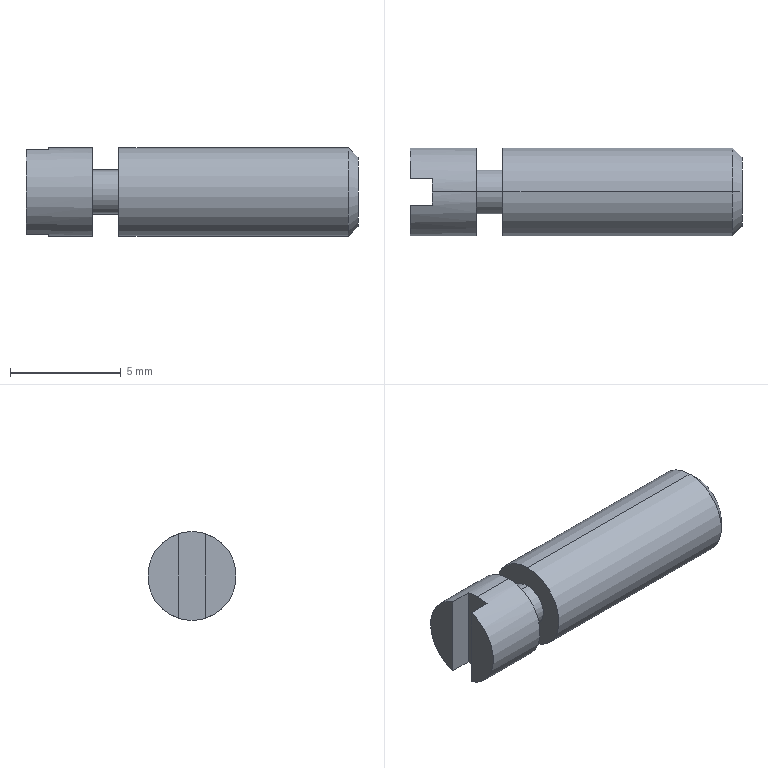Part | STEP file | 11-BSPO4_15b11 | 1 solid | 16 faces | box 15 x 4 x 4 mm | volume 171.383 mm3 | plane 8 | cylinder 6 | cone 2 | commonest cylinder face diameters 4 x4 2 x2
STEP:
#1=CARTESIAN_POINT('',(3.,0.,-2.));
#2=VERTEX_POINT('',#1);
#3=CARTESIAN_POINT('',(3.,0.,2.));
#4=VERTEX_POINT('',#3);
#5=CARTESIAN_POINT('',(3.,0.,0.));
#6=DIRECTION('',(1.,0.,0.));
#7=DIRECTION('',(0.,0.,-1.));
#8=AXIS2_PLACEMENT_3D('',#5,#6,#7);
#9=CIRCLE('',#8,2.);
#10=EDGE_CURVE('',#2,#4,#9,.T.);
#11=ORIENTED_EDGE('',*,*,#10,.F.);
#12=CARTESIAN_POINT('',(1.,0.,-2.));
#13=VERTEX_POINT('',#12);
#14=CARTESIAN_POINT('',(15.,0.,-2.));
#15=DIRECTION('',(-1.,0.,0.));
#16=VECTOR('',#15,1000.);
#17=LINE('',#14,#16);
#18=EDGE_CURVE('',#2,#13,#17,.T.);
#19=ORIENTED_EDGE('',*,*,#18,.T.);
#20=CARTESIAN_POINT('',(1.,0.6,-1.908));
#21=VERTEX_POINT('',#20);
#22=CARTESIAN_POINT('',(1.,0.,0.));
#23=DIRECTION('',(-1.,0.,0.));
#24=DIRECTION('',(0.,0.,1.));
#25=AXIS2_PLACEMENT_3D('',#22,#23,#24);
#26=CIRCLE('',#25,2.);
#27=EDGE_CURVE('',#21,#13,#26,.T.);
#28=ORIENTED_EDGE('',*,*,#27,.F.);
#29=CARTESIAN_POINT('',(0.,0.6,-1.908));
#30=VERTEX_POINT('',#29);
#31=CARTESIAN_POINT('',(15.,0.6,-1.908));
#32=DIRECTION('',(1.,0.,0.));
#33=VECTOR('',#32,1000.);
#34=LINE('',#31,#33);
#35=EDGE_CURVE('',#30,#21,#34,.T.);
#36=ORIENTED_EDGE('',*,*,#35,.F.);
#37=CARTESIAN_POINT('',(0.,0.6,1.908));
#38=VERTEX_POINT('',#37);
#39=CARTESIAN_POINT('',(0.,0.,0.));
#40=DIRECTION('',(-1.,0.,0.));
#41=DIRECTION('',(0.,0.,1.));
#42=AXIS2_PLACEMENT_3D('',#39,#40,#41);
#43=CIRCLE('',#42,2.);
#44=EDGE_CURVE('',#38,#30,#43,.T.);
#45=ORIENTED_EDGE('',*,*,#44,.F.);
#46=CARTESIAN_POINT('',(1.,0.6,1.908));
#47=VERTEX_POINT('',#46);
#48=CARTESIAN_POINT('',(15.,0.6,1.908));
#49=DIRECTION('',(-1.,0.,0.));
#50=VECTOR('',#49,1000.);
#51=LINE('',#48,#50);
#52=EDGE_CURVE('',#47,#38,#51,.T.);
#53=ORIENTED_EDGE('',*,*,#52,.F.);
#54=CARTESIAN_POINT('',(1.,0.,2.));
#55=VERTEX_POINT('',#54);
#56=CARTESIAN_POINT('',(1.,0.,0.));
#57=DIRECTION('',(-1.,0.,0.));
#58=DIRECTION('',(0.,0.,1.));
#59=AXIS2_PLACEMENT_3D('',#56,#57,#58);
#60=CIRCLE('',#59,2.);
#61=EDGE_CURVE('',#55,#47,#60,.T.);
#62=ORIENTED_EDGE('',*,*,#61,.F.);
#63=CARTESIAN_POINT('',(15.,0.,2.));
#64=DIRECTION('',(-1.,0.,0.));
#65=VECTOR('',#64,1000.);
#66=LINE('',#63,#65);
#67=EDGE_CURVE('',#4,#55,#66,.T.);
#68=ORIENTED_EDGE('',*,*,#67,.F.);
#69=EDGE_LOOP('',(#11,#19,#28,#36,#45,#53,#62,#68));
#70=FACE_OUTER_BOUND('',#69,.T.);
#71=CARTESIAN_POINT('',(15.,0.,0.));
#72=DIRECTION('',(-1.,0.,0.));
#73=DIRECTION('',(0.,0.,1.));
#74=AXIS2_PLACEMENT_3D('',#71,#72,#73);
#75=CYLINDRICAL_SURFACE('',#74,2.);
#76=ADVANCED_FACE('',(#70),#75,.T.);
#77=CARTESIAN_POINT('',(4.2,0.,1.));
#78=VERTEX_POINT('',#77);
#79=CARTESIAN_POINT('',(4.2,0.,-1.));
#80=VERTEX_POINT('',#79);
#81=CARTESIAN_POINT('',(4.2,0.,0.));
#82=DIRECTION('',(-1.,0.,0.));
#83=DIRECTION('',(0.,0.,1.));
#84=AXIS2_PLACEMENT_3D('',#81,#82,#83);
#85=CIRCLE('',#84,1.);
#86=EDGE_CURVE('',#78,#80,#85,.T.);
#87=ORIENTED_EDGE('',*,*,#86,.T.);
#88=CARTESIAN_POINT('',(3.,0.,-1.));
#89=VERTEX_POINT('',#88);
#90=CARTESIAN_POINT('',(5.,0.,-1.));
#91=DIRECTION('',(-1.,0.,0.));
#92=VECTOR('',#91,1000.);
#93=LINE('',#90,#92);
#94=EDGE_CURVE('',#80,#89,#93,.T.);
#95=ORIENTED_EDGE('',*,*,#94,.T.);
#96=CARTESIAN_POINT('',(3.,0.,1.));
#97=VERTEX_POINT('',#96);
#98=CARTESIAN_POINT('',(3.,0.,0.));
#99=DIRECTION('',(-1.,0.,0.));
#100=DIRECTION('',(0.,0.,1.));
#101=AXIS2_PLACEMENT_3D('',#98,#99,#100);
#102=CIRCLE('',#101,1.);
#103=EDGE_CURVE('',#97,#89,#102,.T.);
#104=ORIENTED_EDGE('',*,*,#103,.F.);
#105=CARTESIAN_POINT('',(5.,0.,1.));
#106=DIRECTION('',(-1.,0.,0.));
#107=VECTOR('',#106,1000.);
#108=LINE('',#105,#107);
#109=EDGE_CURVE('',#78,#97,#108,.T.);
#110=ORIENTED_EDGE('',*,*,#109,.F.);
#111=EDGE_LOOP('',(#87,#95,#104,#110));
#112=FACE_OUTER_BOUND('',#111,.T.);
#113=CARTESIAN_POINT('',(5.,0.,0.));
#114=DIRECTION('',(-1.,0.,0.));
#115=DIRECTION('',(0.,0.,1.));
#116=AXIS2_PLACEMENT_3D('',#113,#114,#115);
#117=CYLINDRICAL_SURFACE('',#116,1.);
#118=ADVANCED_FACE('',(#112),#117,.T.);
#119=CARTESIAN_POINT('',(15.,0.,1.571));
#120=VERTEX_POINT('',#119);
#121=CARTESIAN_POINT('',(15.,0.,-1.571));
#122=VERTEX_POINT('',#121);
#123=CARTESIAN_POINT('',(15.,0.,0.));
#124=DIRECTION('',(-1.,0.,0.));
#125=DIRECTION('',(0.,0.,1.));
#126=AXIS2_PLACEMENT_3D('',#123,#124,#125);
#127=CIRCLE('',#126,1.571);
#128=EDGE_CURVE('',#120,#122,#127,.T.);
#129=ORIENTED_EDGE('',*,*,#128,.T.);
#130=CARTESIAN_POINT('',(14.571,0.,-2.));
#131=VERTEX_POINT('',#130);
#132=CARTESIAN_POINT('',(15.,0.,-1.571));
#133=DIRECTION('',(-0.7071,0.,-0.7071));
#134=VECTOR('',#133,1000.);
#135=LINE('',#132,#134);
#136=EDGE_CURVE('',#122,#131,#135,.T.);
#137=ORIENTED_EDGE('',*,*,#136,.T.);
#138=CARTESIAN_POINT('',(14.571,0.,2.));
#139=VERTEX_POINT('',#138);
#140=CARTESIAN_POINT('',(14.571,0.,0.));
#141=DIRECTION('',(-1.,0.,0.));
#142=DIRECTION('',(0.,0.,1.));
#143=AXIS2_PLACEMENT_3D('',#140,#141,#142);
#144=CIRCLE('',#143,2.);
#145=EDGE_CURVE('',#139,#131,#144,.T.);
#146=ORIENTED_EDGE('',*,*,#145,.F.);
#147=CARTESIAN_POINT('',(15.,0.,1.571));
#148=DIRECTION('',(-0.7071,0.,0.7071));
#149=VECTOR('',#148,1000.);
#150=LINE('',#147,#149);
#151=EDGE_CURVE('',#120,#139,#150,.T.);
#152=ORIENTED_EDGE('',*,*,#151,.F.);
#153=EDGE_LOOP('',(#129,#137,#146,#152));
#154=FACE_OUTER_BOUND('',#153,.T.);
#155=CARTESIAN_POINT('',(15.,0.,0.));
#156=DIRECTION('',(-1.,0.,0.));
#157=DIRECTION('',(0.,0.,1.));
#158=AXIS2_PLACEMENT_3D('',#155,#156,#157);
#159=CONICAL_SURFACE('',#158,1.571,0.7854);
#160=ADVANCED_FACE('',(#154),#159,.T.);
#161=ORIENTED_EDGE('',*,*,#145,.T.);
#162=CARTESIAN_POINT('',(4.2,0.,-2.));
#163=VERTEX_POINT('',#162);
#164=CARTESIAN_POINT('',(15.,0.,-2.));
#165=DIRECTION('',(-1.,0.,0.));
#166=VECTOR('',#165,1000.);
#167=LINE('',#164,#166);
#168=EDGE_CURVE('',#131,#163,#167,.T.);
#169=ORIENTED_EDGE('',*,*,#168,.T.);
#170=CARTESIAN_POINT('',(4.2,0.,2.));
#171=VERTEX_POINT('',#170);
#172=CARTESIAN_POINT('',(4.2,0.,0.));
#173=DIRECTION('',(-1.,0.,0.));
#174=DIRECTION('',(0.,0.,1.));
#175=AXIS2_PLACEMENT_3D('',#172,#173,#174);
#176=CIRCLE('',#175,2.);
#177=EDGE_CURVE('',#171,#163,#176,.T.);
#178=ORIENTED_EDGE('',*,*,#177,.F.);
#179=CARTESIAN_POINT('',(15.,0.,2.));
#180=DIRECTION('',(-1.,0.,0.));
#181=VECTOR('',#180,1000.);
#182=LINE('',#179,#181);
#183=EDGE_CURVE('',#139,#171,#182,.T.);
#184=ORIENTED_EDGE('',*,*,#183,.F.);
#185=EDGE_LOOP('',(#161,#169,#178,#184));
#186=FACE_OUTER_BOUND('',#185,.T.);
#187=CARTESIAN_POINT('',(15.,0.,0.));
#188=DIRECTION('',(-1.,0.,0.));
#189=DIRECTION('',(0.,0.,1.));
#190=AXIS2_PLACEMENT_3D('',#187,#188,#189);
#191=CYLINDRICAL_SURFACE('',#190,2.);
#192=ADVANCED_FACE('',(#186),#191,.T.);
#193=ORIENTED_EDGE('',*,*,#168,.F.);
#194=CARTESIAN_POINT('',(14.571,0.,0.));
#195=DIRECTION('',(-1.,0.,0.));
#196=DIRECTION('',(0.,0.,1.));
#197=AXIS2_PLACEMENT_3D('',#194,#195,#196);
#198=CIRCLE('',#197,2.);
#199=EDGE_CURVE('',#131,#139,#198,.T.);
#200=ORIENTED_EDGE('',*,*,#199,.T.);
#201=ORIENTED_EDGE('',*,*,#183,.T.);
#202=CARTESIAN_POINT('',(4.2,0.,0.));
#203=DIRECTION('',(-1.,0.,0.));
#204=DIRECTION('',(0.,0.,1.));
#205=AXIS2_PLACEMENT_3D('',#202,#203,#204);
#206=CIRCLE('',#205,2.);
#207=EDGE_CURVE('',#163,#171,#206,.T.);
#208=ORIENTED_EDGE('',*,*,#207,.F.);
#209=EDGE_LOOP('',(#193,#200,#201,#208));
#210=FACE_OUTER_BOUND('',#209,.T.);
#211=CARTESIAN_POINT('',(15.,0.,0.));
#212=DIRECTION('',(-1.,0.,0.));
#213=DIRECTION('',(0.,0.,1.));
#214=AXIS2_PLACEMENT_3D('',#211,#212,#213);
#215=CYLINDRICAL_SURFACE('',#214,2.);
#216=ADVANCED_FACE('',(#210),#215,.T.);
#217=ORIENTED_EDGE('',*,*,#136,.F.);
#218=CARTESIAN_POINT('',(15.,0.,0.));
#219=DIRECTION('',(-1.,0.,0.));
#220=DIRECTION('',(0.,0.,1.));
#221=AXIS2_PLACEMENT_3D('',#218,#219,#220);
#222=CIRCLE('',#221,1.571);
#223=EDGE_CURVE('',#122,#120,#222,.T.);
#224=ORIENTED_EDGE('',*,*,#223,.T.);
#225=ORIENTED_EDGE('',*,*,#151,.T.);
#226=ORIENTED_EDGE('',*,*,#199,.F.);
#227=EDGE_LOOP('',(#217,#224,#225,#226));
#228=FACE_OUTER_BOUND('',#227,.T.);
#229=CARTESIAN_POINT('',(15.,0.,0.));
#230=DIRECTION('',(-1.,0.,0.));
#231=DIRECTION('',(0.,0.,1.));
#232=AXIS2_PLACEMENT_3D('',#229,#230,#231);
#233=CONICAL_SURFACE('',#232,1.571,0.7854);
#234=ADVANCED_FACE('',(#228),#233,.T.);
#235=ORIENTED_EDGE('',*,*,#128,.F.);
#236=ORIENTED_EDGE('',*,*,#223,.F.);
#237=EDGE_LOOP('',(#235,#236));
#238=FACE_OUTER_BOUND('',#237,.T.);
#239=CARTESIAN_POINT('',(15.,1.571,0.));
#240=DIRECTION('',(-1.,0.,0.));
#241=DIRECTION('',(0.,0.,1.));
#242=AXIS2_PLACEMENT_3D('',#239,#240,#241);
#243=PLANE('',#242);
#244=ADVANCED_FACE('',(#238),#243,.F.);
#245=ORIENTED_EDGE('',*,*,#103,.T.);
#246=CARTESIAN_POINT('',(3.,0.,0.));
#247=DIRECTION('',(-1.,0.,0.));
#248=DIRECTION('',(0.,0.,1.));
#249=AXIS2_PLACEMENT_3D('',#246,#247,#248);
#250=CIRCLE('',#249,1.);
#251=EDGE_CURVE('',#89,#97,#250,.T.);
#252=ORIENTED_EDGE('',*,*,#251,.T.);
#253=EDGE_LOOP('',(#245,#252));
#254=FACE_BOUND('',#253,.T.);
#255=CARTESIAN_POINT('',(3.,0.,0.));
#256=DIRECTION('',(1.,0.,0.));
#257=DIRECTION('',(0.,0.,-1.));
#258=AXIS2_PLACEMENT_3D('',#255,#256,#257);
#259=CIRCLE('',#258,2.);
#260=EDGE_CURVE('',#4,#2,#259,.T.);
#261=ORIENTED_EDGE('',*,*,#260,.T.);
#262=ORIENTED_EDGE('',*,*,#10,.T.);
#263=EDGE_LOOP('',(#261,#262));
#264=FACE_OUTER_BOUND('',#263,.T.);
#265=CARTESIAN_POINT('',(3.,2.2,0.));
#266=DIRECTION('',(1.,0.,0.));
#267=DIRECTION('',(0.,0.,-1.));
#268=AXIS2_PLACEMENT_3D('',#265,#266,#267);
#269=PLANE('',#268);
#270=ADVANCED_FACE('',(#254,#264),#269,.T.);
#271=ORIENTED_EDGE('',*,*,#86,.F.);
#272=CARTESIAN_POINT('',(4.2,0.,0.));
#273=DIRECTION('',(-1.,0.,0.));
#274=DIRECTION('',(0.,0.,1.));
#275=AXIS2_PLACEMENT_3D('',#272,#273,#274);
#276=CIRCLE('',#275,1.);
#277=EDGE_CURVE('',#80,#78,#276,.T.);
#278=ORIENTED_EDGE('',*,*,#277,.F.);
#279=EDGE_LOOP('',(#271,#278));
#280=FACE_BOUND('',#279,.T.);
#281=ORIENTED_EDGE('',*,*,#177,.T.);
#282=ORIENTED_EDGE('',*,*,#207,.T.);
#283=EDGE_LOOP('',(#281,#282));
#284=FACE_OUTER_BOUND('',#283,.T.);
#285=CARTESIAN_POINT('',(4.2,1.,0.));
#286=DIRECTION('',(-1.,0.,0.));
#287=DIRECTION('',(0.,0.,1.));
#288=AXIS2_PLACEMENT_3D('',#285,#286,#287);
#289=PLANE('',#288);
#290=ADVANCED_FACE('',(#280,#284),#289,.T.);
#291=ORIENTED_EDGE('',*,*,#94,.F.);
#292=ORIENTED_EDGE('',*,*,#277,.T.);
#293=ORIENTED_EDGE('',*,*,#109,.T.);
#294=ORIENTED_EDGE('',*,*,#251,.F.);
#295=EDGE_LOOP('',(#291,#292,#293,#294));
#296=FACE_OUTER_BOUND('',#295,.T.);
#297=CARTESIAN_POINT('',(5.,0.,0.));
#298=DIRECTION('',(-1.,0.,0.));
#299=DIRECTION('',(0.,0.,1.));
#300=AXIS2_PLACEMENT_3D('',#297,#298,#299);
#301=CYLINDRICAL_SURFACE('',#300,1.);
#302=ADVANCED_FACE('',(#296),#301,.T.);
#303=CARTESIAN_POINT('',(0.,0.6,2.));
#304=DIRECTION('',(0.,0.,-1.));
#305=VECTOR('',#304,1000.);
#306=LINE('',#303,#305);
#307=EDGE_CURVE('',#38,#30,#306,.T.);
#308=ORIENTED_EDGE('',*,*,#307,.F.);
#309=ORIENTED_EDGE('',*,*,#44,.T.);
#310=EDGE_LOOP('',(#308,#309));
#311=FACE_OUTER_BOUND('',#310,.T.);
#312=CARTESIAN_POINT('',(0.,0.,0.));
#313=DIRECTION('',(1.,0.,0.));
#314=DIRECTION('',(0.,0.,-1.));
#315=AXIS2_PLACEMENT_3D('',#312,#313,#314);
#316=PLANE('',#315);
#317=ADVANCED_FACE('',(#311),#316,.F.);
#318=CARTESIAN_POINT('',(0.,-0.6,1.908));
#319=VERTEX_POINT('',#318);
#320=CARTESIAN_POINT('',(0.,-0.6,-1.908));
#321=VERTEX_POINT('',#320);
#322=CARTESIAN_POINT('',(0.,-0.6,2.));
#323=DIRECTION('',(0.,0.,-1.));
#324=VECTOR('',#323,1000.);
#325=LINE('',#322,#324);
#326=EDGE_CURVE('',#319,#321,#325,.T.);
#327=ORIENTED_EDGE('',*,*,#326,.T.);
#328=CARTESIAN_POINT('',(0.,0.,0.));
#329=DIRECTION('',(-1.,0.,0.));
#330=DIRECTION('',(0.,0.,1.));
#331=AXIS2_PLACEMENT_3D('',#328,#329,#330);
#332=CIRCLE('',#331,2.);
#333=EDGE_CURVE('',#321,#319,#332,.T.);
#334=ORIENTED_EDGE('',*,*,#333,.T.);
#335=EDGE_LOOP('',(#327,#334));
#336=FACE_OUTER_BOUND('',#335,.T.);
#337=CARTESIAN_POINT('',(0.,0.,0.));
#338=DIRECTION('',(1.,0.,0.));
#339=DIRECTION('',(0.,0.,-1.));
#340=AXIS2_PLACEMENT_3D('',#337,#338,#339);
#341=PLANE('',#340);
#342=ADVANCED_FACE('',(#336),#341,.F.);
#343=CARTESIAN_POINT('',(1.,-0.6,-1.908));
#344=VERTEX_POINT('',#343);
#345=CARTESIAN_POINT('',(15.,-0.6,-1.908));
#346=DIRECTION('',(-1.,0.,0.));
#347=VECTOR('',#346,1000.);
#348=LINE('',#345,#347);
#349=EDGE_CURVE('',#344,#321,#348,.T.);
#350=ORIENTED_EDGE('',*,*,#349,.T.);
#351=ORIENTED_EDGE('',*,*,#326,.F.);
#352=CARTESIAN_POINT('',(1.,-0.6,1.908));
#353=VERTEX_POINT('',#352);
#354=CARTESIAN_POINT('',(15.,-0.6,1.908));
#355=DIRECTION('',(1.,0.,0.));
#356=VECTOR('',#355,1000.);
#357=LINE('',#354,#356);
#358=EDGE_CURVE('',#319,#353,#357,.T.);
#359=ORIENTED_EDGE('',*,*,#358,.T.);
#360=CARTESIAN_POINT('',(1.,-0.6,2.));
#361=DIRECTION('',(0.,0.,-1.));
#362=VECTOR('',#361,1000.);
#363=LINE('',#360,#362);
#364=EDGE_CURVE('',#353,#344,#363,.T.);
#365=ORIENTED_EDGE('',*,*,#364,.T.);
#366=EDGE_LOOP('',(#350,#351,#359,#365));
#367=FACE_OUTER_BOUND('',#366,.T.);
#368=CARTESIAN_POINT('',(0.,-0.6,2.));
#369=DIRECTION('',(0.,1.,0.));
#370=DIRECTION('',(0.,0.,1.));
#371=AXIS2_PLACEMENT_3D('',#368,#369,#370);
#372=PLANE('',#371);
#373=ADVANCED_FACE('',(#367),#372,.T.);
#374=CARTESIAN_POINT('',(1.,0.6,2.));
#375=DIRECTION('',(0.,0.,-1.));
#376=VECTOR('',#375,1000.);
#377=LINE('',#374,#376);
#378=EDGE_CURVE('',#47,#21,#377,.T.);
#379=ORIENTED_EDGE('',*,*,#378,.T.);
#380=ORIENTED_EDGE('',*,*,#27,.T.);
#381=CARTESIAN_POINT('',(1.,0.,0.));
#382=DIRECTION('',(-1.,0.,0.));
#383=DIRECTION('',(0.,0.,1.));
#384=AXIS2_PLACEMENT_3D('',#381,#382,#383);
#385=CIRCLE('',#384,2.);
#386=EDGE_CURVE('',#13,#344,#385,.T.);
#387=ORIENTED_EDGE('',*,*,#386,.T.);
#388=ORIENTED_EDGE('',*,*,#364,.F.);
#389=CARTESIAN_POINT('',(1.,0.,0.));
#390=DIRECTION('',(-1.,0.,0.));
#391=DIRECTION('',(0.,0.,1.));
#392=AXIS2_PLACEMENT_3D('',#389,#390,#391);
#393=CIRCLE('',#392,2.);
#394=EDGE_CURVE('',#353,#55,#393,.T.);
#395=ORIENTED_EDGE('',*,*,#394,.T.);
#396=ORIENTED_EDGE('',*,*,#61,.T.);
#397=EDGE_LOOP('',(#379,#380,#387,#388,#395,#396));
#398=FACE_OUTER_BOUND('',#397,.T.);
#399=CARTESIAN_POINT('',(1.,-0.6,2.));
#400=DIRECTION('',(-1.,0.,0.));
#401=DIRECTION('',(0.,0.,1.));
#402=AXIS2_PLACEMENT_3D('',#399,#400,#401);
#403=PLANE('',#402);
#404=ADVANCED_FACE('',(#398),#403,.T.);
#405=ORIENTED_EDGE('',*,*,#52,.T.);
#406=ORIENTED_EDGE('',*,*,#307,.T.);
#407=ORIENTED_EDGE('',*,*,#35,.T.);
#408=ORIENTED_EDGE('',*,*,#378,.F.);
#409=EDGE_LOOP('',(#405,#406,#407,#408));
#410=FACE_OUTER_BOUND('',#409,.T.);
#411=CARTESIAN_POINT('',(1.,0.6,2.));
#412=DIRECTION('',(0.,-1.,0.));
#413=DIRECTION('',(0.,0.,-1.));
#414=AXIS2_PLACEMENT_3D('',#411,#412,#413);
#415=PLANE('',#414);
#416=ADVANCED_FACE('',(#410),#415,.T.);
#417=ORIENTED_EDGE('',*,*,#18,.F.);
#418=ORIENTED_EDGE('',*,*,#260,.F.);
#419=ORIENTED_EDGE('',*,*,#67,.T.);
#420=ORIENTED_EDGE('',*,*,#394,.F.);
#421=ORIENTED_EDGE('',*,*,#358,.F.);
#422=ORIENTED_EDGE('',*,*,#333,.F.);
#423=ORIENTED_EDGE('',*,*,#349,.F.);
#424=ORIENTED_EDGE('',*,*,#386,.F.);
#425=EDGE_LOOP('',(#417,#418,#419,#420,#421,#422,#423,#424));
#426=FACE_OUTER_BOUND('',#425,.T.);
#427=CARTESIAN_POINT('',(15.,0.,0.));
#428=DIRECTION('',(-1.,0.,0.));
#429=DIRECTION('',(0.,0.,1.));
#430=AXIS2_PLACEMENT_3D('',#427,#428,#429);
#431=CYLINDRICAL_SURFACE('',#430,2.);
#432=ADVANCED_FACE('',(#426),#431,.T.);
#433=CLOSED_SHELL('',(#76,#118,#160,#192,#216,#234,#244,#270,#290,#302,#317,#342,#373,#404,#416,#432));
#434=MANIFOLD_SOLID_BREP('',#433);
#435=CARTESIAN_POINT('',(0.,0.,0.));
#436=DIRECTION('',(0.,0.,1.));
#437=DIRECTION('',(1.,0.,0.));
#438=AXIS2_PLACEMENT_3D('',#435,#436,#437);
#439=(LENGTH_UNIT()NAMED_UNIT(*)SI_UNIT(.MILLI.,.METRE.));
#440=UNCERTAINTY_MEASURE_WITH_UNIT(LENGTH_MEASURE(0.00001),#439,'','');
#441=(NAMED_UNIT(*)PLANE_ANGLE_UNIT()SI_UNIT($,.RADIAN.));
#442=(NAMED_UNIT(*)SI_UNIT($,.STERADIAN.)SOLID_ANGLE_UNIT());
#443=(GEOMETRIC_REPRESENTATION_CONTEXT(3)GLOBAL_UNCERTAINTY_ASSIGNED_CONTEXT((#440))GLOBAL_UNIT_ASSIGNED_CONTEXT((#439,#441,#442))REPRESENTATION_CONTEXT('',''));
#444=ADVANCED_BREP_SHAPE_REPRESENTATION('',(#434,#438),#443);